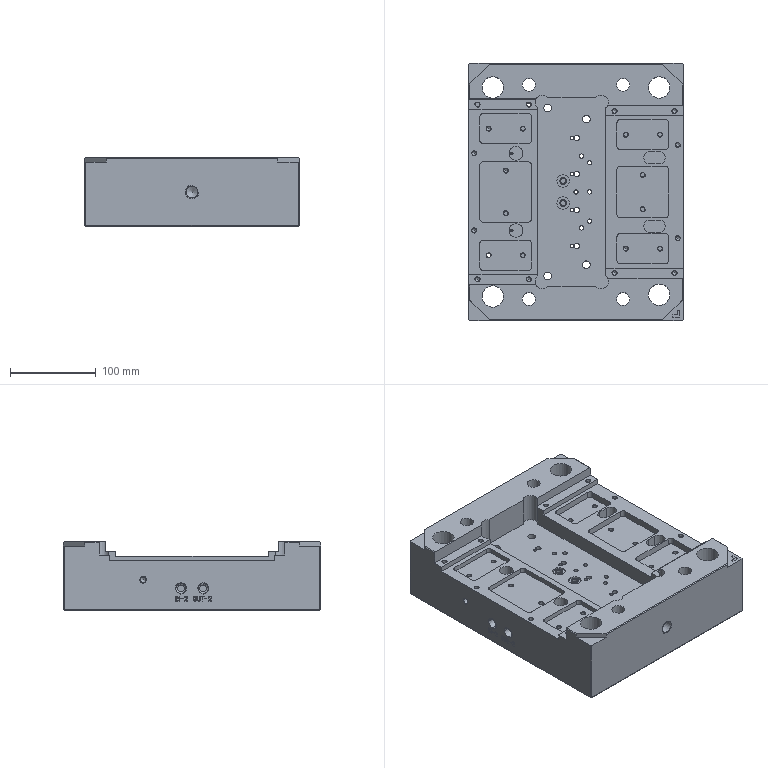NC program | PowerMill | posted with a generic post | part box 250 x 300 x 80 mm
Whole program:
%
O0001
N104 ( POWERMILL CB  : 2026004.0)
N105 ( POST VER      : 2026.0.0.5161)
N106 ( OPTION FILE   : FANUC)
N107 ( OUTPUT WORKPLANE : 1)
N108 (  )
N109 ( TOOL LIST )
N110 (-----------------------------------)
N111 ( NO. | ID    | DIA.| TIP RAD|LENGTH)
N112 (-----------------------------------)
N113 (    1|￠4_1_1| 4.0 |  0.0   |139.2 )
N114 (-----------------------------------)
N115 (  )
N116 ( NUMBER OF TOOLPATHS: 1.0 )
N117 ( ESTIMATED PROGRAM DURATION: 0 HOURS 5 MIN 16 SEC)
N118 (  )
N119 G00 G21 G80 G40 G17
N120 G90
N121 G54
N122 G53 Z0.0
N123 (---------------)
N124 ( START TOOLPATH : 31开粗-￠4-钻孔加工 )
N125 (---------------)
N126 ( TOOL NO.    :1 )
N127 ( TOOL TYPE   : DRILL)
N128 ( TOOL ID     : ￠4_1_1)
N129 ( TOOL DIA    : 4.0 LENGTH 139.2)
N130 T1
N131 M6
N132 S800 M03
N133 G00 G90 X63.0 Y4.6
N134 G43 Z20.0 H1
N135
N136 G05 P10000 R8
N137 Z11.0
N138 G01 Z-1.0 F60.0
N139 G00 Z11.0
N140 Z-0.6
N141 G01 Z-3.0
N142 G00 Z11.0
N143 Z-2.6
N144 G01 Z-5.0
N145 G00 Z11.0
N146 Z-4.6
N147 G01 Z-7.0
N148 G00 Z11.0
N149 Z-6.6
N150 G01 Z-9.0
N151 G00 Z11.0
N152 Z-8.6
N153 G01 Z-11.0
N154 G00 Z11.0
N155 Z-10.6
N156 G01 Z-13.0
N157 G00 Z11.0
N158 Z-12.6
N159 G01 Z-15.0
N160 G00 Z11.0
N161 Z-14.6
N162 G01 Z-17.0
N163 G00 Z11.0
N164 Z-16.6
N165 G01 Z-19.0
N166 G00 Z11.0
N167 Z-18.6
N168 G01 Z-21.0
N169 G00 Z11.0
N170 Z-20.6
N171 G01 Z-23.0
N172 G00 Z11.0
N173 Z-22.6
N174 G01 Z-25.0
N175 G00 Z11.0
N176 Z-24.6
N177 G01 Z-27.0
N178 G00 Z11.0
N179 Z-26.6
N180 G01 Z-29.0
N181 G00 Z11.0
N182 Z-28.6
N183 G01 Z-31.0
N184 G00 Z11.0
N185 Z-30.6
N186 G01 Z-33.0
N187 G00 Z11.0
N188 Z-32.6
N189 G01 Z-35.0
N190 G00 Z11.0
N191 Z-34.6
N192 G01 Z-37.0
N193 G00 Z11.0
N194 Z-36.6
N195 G01 Z-39.0
N196 G00 Z11.0
N197 Z-38.6
N198 G01 Z-41.0
N199 G00 Z11.0
N200 Z-40.6
N201 G01 Z-43.0
N202 G00 Z11.0
N203 Z-42.6
N204 G01 Z-45.0
N205 G00 Z11.0
N206 Z-44.6
N207 G01 Z-47.0
N208 G00 Z11.0
N209 Z-46.6
N210 G01 Z-47.9557
N211 G00 Z20.0
N212 X21.0
N213 Z11.0
N214 G01 Z-1.0
N215 G00 Z11.0
N216 Z-0.6
N217 G01 Z-3.0
N218 G00 Z11.0
N219 Z-2.6
N220 G01 Z-5.0
N221 G00 Z11.0
N222 Z-4.6
N223 G01 Z-7.0
N224 G00 Z11.0
N225 Z-6.6
N226 G01 Z-9.0
N227 G00 Z11.0
N228 Z-8.6
N229 G01 Z-11.0
N230 G00 Z11.0
N231 Z-10.6
N232 G01 Z-13.0
N233 G00 Z11.0
N234 Z-12.6
N235 G01 Z-15.0
N236 G00 Z11.0
N237 Z-14.6
N238 G01 Z-17.0
N239 G00 Z11.0
N240 Z-16.6
N241 G01 Z-19.0
N242 G00 Z11.0
N243 Z-18.6
N244 G01 Z-21.0
N245 G00 Z11.0
N246 Z-20.6
N247 G01 Z-23.0
N248 G00 Z11.0
N249 Z-22.6
N250 G01 Z-25.0
N251 G00 Z11.0
N252 Z-24.6
N253 G01 Z-27.0
N254 G00 Z11.0
N255 Z-26.6
N256 G01 Z-29.0
N257 G00 Z11.0
N258 Z-28.6
N259 G01 Z-31.0
N260 G00 Z11.0
N261 Z-30.6
N262 G01 Z-33.0
N263 G00 Z11.0
N264 Z-32.6
N265 G01 Z-35.0
N266 G00 Z11.0
N267 Z-34.6
N268 G01 Z-37.0
N269 G00 Z11.0
N270 Z-36.6
N271 G01 Z-39.0
N272 G00 Z11.0
N273 Z-38.6
N274 G01 Z-41.0
N275 G00 Z11.0
N276 Z-40.6
N277 G01 Z-43.0
N278 G00 Z11.0
N279 Z-42.6
N280 G01 Z-45.0
N281 G00 Z11.0
N282 Z-44.6
N283 G01 Z-47.0
N284 G00 Z11.0
N285 Z-46.6
N286 G01 Z-47.9557
N287 G00 Z20.0
N288 X-21.0
N289 Z11.0
N290 G01 Z-1.0
N291 G00 Z11.0
N292 Z-0.6
N293 G01 Z-3.0
N294 G00 Z11.0
N295 Z-2.6
N296 G01 Z-5.0
N297 G00 Z11.0
N298 Z-4.6
N299 G01 Z-7.0
N300 G00 Z11.0
N301 Z-6.6
N302 G01 Z-9.0
N303 G00 Z11.0
N304 Z-8.6
N305 G01 Z-11.0
N306 G00 Z11.0
N307 Z-10.6
N308 G01 Z-13.0
N309 G00 Z11.0
N310 Z-12.6
N311 G01 Z-15.0
N312 G00 Z11.0
N313 Z-14.6
N314 G01 Z-17.0
N315 G00 Z11.0
N316 Z-16.6
N317 G01 Z-19.0
N318 G00 Z11.0
N319 Z-18.6
N320 G01 Z-21.0
N321 G00 Z11.0
N322 Z-20.6
N323 G01 Z-23.0
N324 G00 Z11.0
N325 Z-22.6
N326 G01 Z-25.0
N327 G00 Z11.0
N328 Z-24.6
N329 G01 Z-27.0
N330 G00 Z11.0
N331 Z-26.6
N332 G01 Z-29.0
N333 G00 Z11.0
N334 Z-28.6
N335 G01 Z-31.0
N336 G00 Z11.0
N337 Z-30.6
N338 G01 Z-33.0
N339 G00 Z11.0
N340 Z-32.6
N341 G01 Z-35.0
N342 G00 Z11.0
N343 Z-34.6
N344 G01 Z-37.0
N345 G00 Z11.0
N346 Z-36.6
N347 G01 Z-39.0
N348 G00 Z11.0
N349 Z-38.6
N350 G01 Z-41.0
N351 G00 Z11.0
N352 Z-40.6
N353 G01 Z-43.0
N354 G00 Z11.0
N355 Z-42.6
N356 G01 Z-45.0
N357 G00 Z11.0
N358 Z-44.6
N359 G01 Z-47.0
N360 G00 Z11.0
N361 Z-46.6
N362 G01 Z-47.9557
N363 G00 Z20.0
N364 X-63.0
N365 Z11.0
N366 G01 Z-1.0
N367 G00 Z11.0
N368 Z-0.6
N369 G01 Z-3.0
N370 G00 Z11.0
N371 Z-2.6
N372 G01 Z-5.0
N373 G00 Z11.0
N374 Z-4.6
N375 G01 Z-7.0
N376 G00 Z11.0
N377 Z-6.6
N378 G01 Z-9.0
N379 G00 Z11.0
N380 Z-8.6
N381 G01 Z-11.0
N382 G00 Z11.0
N383 Z-10.6
N384 G01 Z-13.0
N385 G00 Z11.0
N386 Z-12.6
N387 G01 Z-15.0
N388 G00 Z11.0
N389 Z-14.6
N390 G01 Z-17.0
N391 G00 Z11.0
N392 Z-16.6
N393 G01 Z-19.0
N394 G00 Z11.0
N395 Z-18.6
N396 G01 Z-21.0
N397 G00 Z11.0
N398 Z-20.6
N399 G01 Z-23.0
N400 G00 Z11.0
N401 Z-22.6
N402 G01 Z-25.0
N403 G00 Z11.0
N404 Z-24.6
N405 G01 Z-27.0
N406 G00 Z11.0
N407 Z-26.6
N408 G01 Z-29.0
N409 G00 Z11.0
N410 Z-28.6
N411 G01 Z-31.0
N412 G00 Z11.0
N413 Z-30.6
N414 G01 Z-33.0
N415 G00 Z11.0
N416 Z-32.6
N417 G01 Z-35.0
N418 G00 Z11.0
N419 Z-34.6
N420 G01 Z-37.0
N421 G00 Z11.0
N422 Z-36.6
N423 G01 Z-39.0
N424 G00 Z11.0
N425 Z-38.6
N426 G01 Z-41.0
N427 G00 Z11.0
N428 Z-40.6
N429 G01 Z-43.0
N430 G00 Z11.0
N431 Z-42.6
N432 G01 Z-45.0
N433 G00 Z11.0
N434 Z-44.6
N435 G01 Z-47.0
N436 G00 Z11.0
N437 Z-46.6
N438 G01 Z-47.9557
N439 G00 Z20.0
N440 G05 P0
N441 (---------------)
N442 ( END TOOLPATH : 31开粗-￠4-钻孔加工 )
N443 (---------------)
N444
N445 M05
N446 G53 Z0.0
N447 M30
%